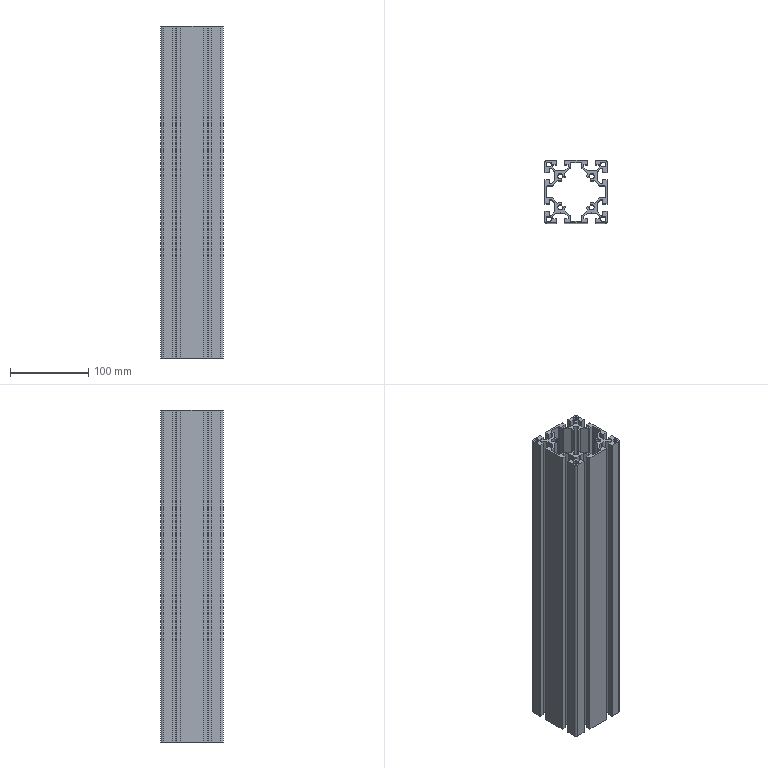Part | SolidWorks | features BaseBody 1 | 1 solid | 231 faces | box 80 x 80 x 425 mm | volume 723822 mm3 | plane 154 | cylinder 77 | commonest cylinder face diameters 2 x34 0.6 x17 6.8 x12 12 x10 6 x4